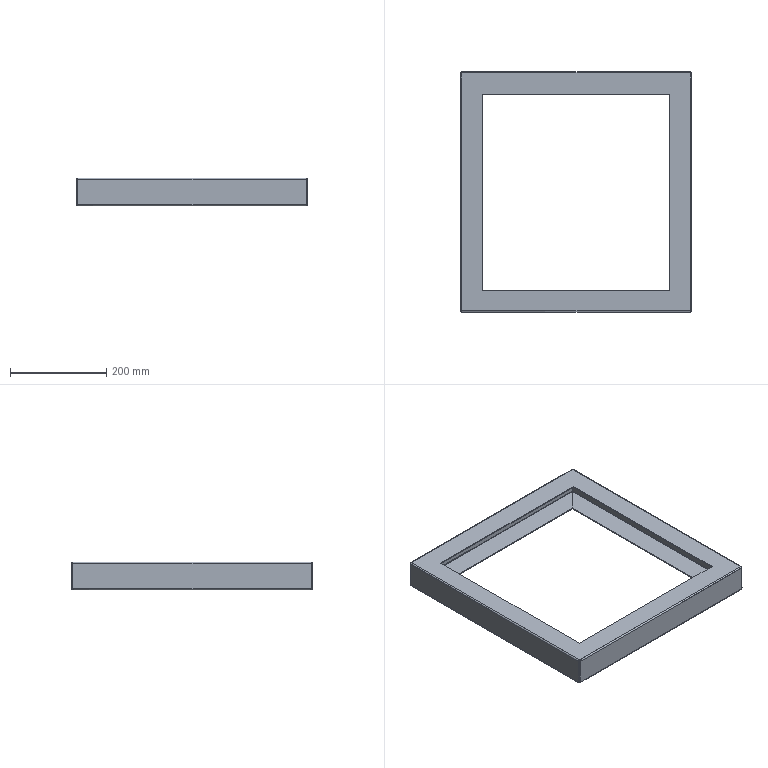Part | SolidWorks | features FlatPattern 1, ICE 1, SMBaseFlange 1, SMMiteredFlange 1, SheetMetal 1 | 1 solid | 74 faces | box 480 x 500 x 58 mm | volume 526033 mm3 | plane 42 | spline 16 | cylinder 16 | commonest cylinder face diameters 1.473 x8 5.473 x8